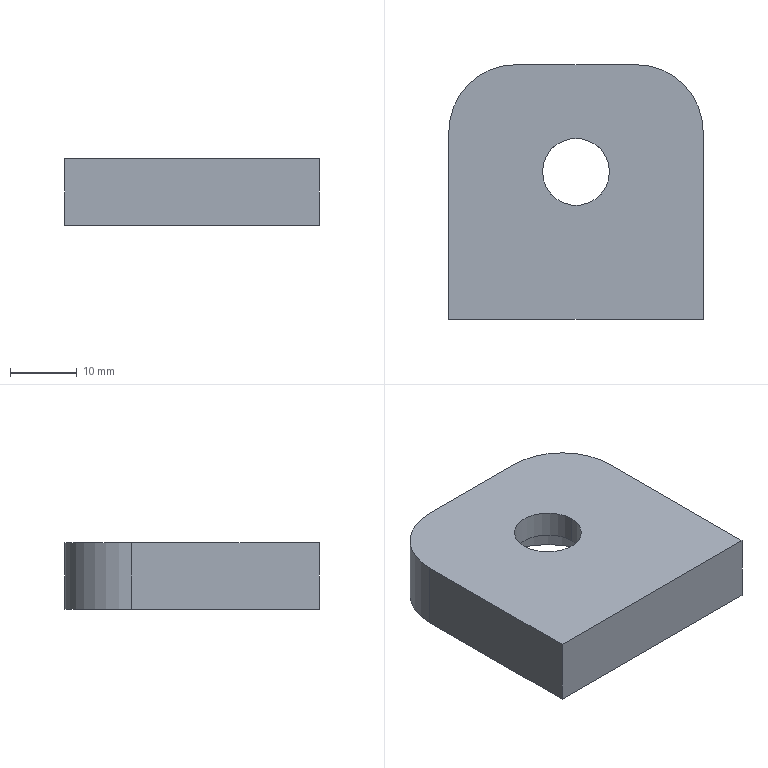Part | STEP file | Fixed block QY-1-06 | 1 solid | 13 faces | box 38 x 38 x 10 mm | volume 11416 mm3 | plane 7 | cylinder 6 | commonest cylinder face diameters 10 x2 20 x2 22 x2
STEP:
#1=CARTESIAN_POINT('',(0.,0.,0.));
#2=DIRECTION('',(0.,0.,1.));
#3=DIRECTION('',(1.,0.,0.));
#4=AXIS2_PLACEMENT_3D('',#1,#2,#3);
#5=CARTESIAN_POINT('',(-11.,3.,6.));
#6=VERTEX_POINT('',#5);
#7=CARTESIAN_POINT('',(-11.,3.,0.));
#8=VERTEX_POINT('',#7);
#9=CARTESIAN_POINT('',(-11.,3.,6.));
#10=DIRECTION('',(0.,0.,-1.));
#11=VECTOR('',#10,1.);
#12=LINE('',#9,#11);
#13=CARTESIAN_POINT('',(0.,3.,6.));
#14=DIRECTION('',(0.,0.,-1.));
#15=DIRECTION('',(-1.,0.,0.));
#16=AXIS2_PLACEMENT_3D('',#13,#14,#15);
#17=CYLINDRICAL_SURFACE('',#16,11.);
#18=CARTESIAN_POINT('',(6.283,0.));
#19=DIRECTION('',(0.,1.));
#20=VECTOR('',#19,1.);
#21=LINE('',#18,#20);
#22=(GEOMETRIC_REPRESENTATION_CONTEXT(2)PARAMETRIC_REPRESENTATION_CONTEXT()REPRESENTATION_CONTEXT('',''));
#23=DEFINITIONAL_REPRESENTATION('',(#21),#22);
#24=PCURVE('',#17,#23);
#25=CARTESIAN_POINT('',(0.,3.,6.));
#26=DIRECTION('',(0.,0.,-1.));
#27=DIRECTION('',(-1.,0.,0.));
#28=AXIS2_PLACEMENT_3D('',#25,#26,#27);
#29=CYLINDRICAL_SURFACE('',#28,11.);
#30=CARTESIAN_POINT('',(0.,0.));
#31=DIRECTION('',(0.,1.));
#32=VECTOR('',#31,1.);
#33=LINE('',#30,#32);
#34=(GEOMETRIC_REPRESENTATION_CONTEXT(2)PARAMETRIC_REPRESENTATION_CONTEXT()REPRESENTATION_CONTEXT('',''));
#35=DEFINITIONAL_REPRESENTATION('',(#33),#34);
#36=PCURVE('',#29,#35);
#37=SURFACE_CURVE('',#12,(#24,#36),.PCURVE_S1.);
#38=EDGE_CURVE('',#6,#8,#37,.T.);
#39=ORIENTED_EDGE('',*,*,#38,.T.);
#40=CARTESIAN_POINT('',(11.,3.,0.));
#41=VERTEX_POINT('',#40);
#42=CARTESIAN_POINT('',(0.,3.,0.));
#43=DIRECTION('',(0.,0.,-1.));
#44=DIRECTION('',(-1.,0.,0.));
#45=AXIS2_PLACEMENT_3D('',#42,#43,#44);
#46=CIRCLE('',#45,11.);
#47=CARTESIAN_POINT('',(0.,6.));
#48=DIRECTION('',(1.,0.));
#49=VECTOR('',#48,1.);
#50=LINE('',#47,#49);
#51=(GEOMETRIC_REPRESENTATION_CONTEXT(2)PARAMETRIC_REPRESENTATION_CONTEXT()REPRESENTATION_CONTEXT('',''));
#52=DEFINITIONAL_REPRESENTATION('',(#50),#51);
#53=PCURVE('',#17,#52);
#54=CARTESIAN_POINT('',(-9.,9.,0.));
#55=DIRECTION('',(0.,0.,1.));
#56=DIRECTION('',(1.,0.,0.));
#57=AXIS2_PLACEMENT_3D('',#54,#55,#56);
#58=PLANE('',#57);
#59=CARTESIAN_POINT('',(-2.,-6.));
#60=CARTESIAN_POINT('',(-2.,13.053));
#61=CARTESIAN_POINT('',(14.5,3.526));
#62=CARTESIAN_POINT('',(31.,-6.));
#63=CARTESIAN_POINT('',(14.5,-15.526));
#64=CARTESIAN_POINT('',(-2.,-25.053));
#65=CARTESIAN_POINT('',(-2.,-6.));
#66=(BOUNDED_CURVE()B_SPLINE_CURVE(2,(#59,#60,#61,#62,#63,#64,#65),.UNSPECIFIED.,.T.,.F.)B_SPLINE_CURVE_WITH_KNOTS((1,2,2,2,2,1),(-2.094,0.,2.094,4.189,6.283,8.378),.UNSPECIFIED.)CURVE()GEOMETRIC_REPRESENTATION_ITEM()RATIONAL_B_SPLINE_CURVE((1.,0.5,1.,0.5,1.,0.5,1.))REPRESENTATION_ITEM(''));
#67=(GEOMETRIC_REPRESENTATION_CONTEXT(2)PARAMETRIC_REPRESENTATION_CONTEXT()REPRESENTATION_CONTEXT('',''));
#68=DEFINITIONAL_REPRESENTATION('',(#66),#67);
#69=PCURVE('',#58,#68);
#70=SURFACE_CURVE('',#46,(#53,#69),.PCURVE_S1.);
#71=EDGE_CURVE('',#41,#8,#70,.T.);
#72=ORIENTED_EDGE('',*,*,#71,.F.);
#73=CARTESIAN_POINT('',(11.,3.,6.));
#74=VERTEX_POINT('',#73);
#75=CARTESIAN_POINT('',(11.,3.,6.));
#76=DIRECTION('',(0.,0.,-1.));
#77=VECTOR('',#76,1.);
#78=LINE('',#75,#77);
#79=CARTESIAN_POINT('',(3.142,0.));
#80=DIRECTION('',(0.,1.));
#81=VECTOR('',#80,1.);
#82=LINE('',#79,#81);
#83=(GEOMETRIC_REPRESENTATION_CONTEXT(2)PARAMETRIC_REPRESENTATION_CONTEXT()REPRESENTATION_CONTEXT('',''));
#84=DEFINITIONAL_REPRESENTATION('',(#82),#83);
#85=PCURVE('',#17,#84);
#86=CARTESIAN_POINT('',(3.142,0.));
#87=DIRECTION('',(0.,1.));
#88=VECTOR('',#87,1.);
#89=LINE('',#86,#88);
#90=(GEOMETRIC_REPRESENTATION_CONTEXT(2)PARAMETRIC_REPRESENTATION_CONTEXT()REPRESENTATION_CONTEXT('',''));
#91=DEFINITIONAL_REPRESENTATION('',(#89),#90);
#92=PCURVE('',#29,#91);
#93=SURFACE_CURVE('',#78,(#85,#92),.PCURVE_S1.);
#94=EDGE_CURVE('',#74,#41,#93,.T.);
#95=ORIENTED_EDGE('',*,*,#94,.F.);
#96=CARTESIAN_POINT('',(0.,3.,6.));
#97=DIRECTION('',(0.,0.,-1.));
#98=DIRECTION('',(-1.,0.,0.));
#99=AXIS2_PLACEMENT_3D('',#96,#97,#98);
#100=CIRCLE('',#99,11.);
#101=CARTESIAN_POINT('',(0.,0.));
#102=DIRECTION('',(1.,0.));
#103=VECTOR('',#102,1.);
#104=LINE('',#101,#103);
#105=(GEOMETRIC_REPRESENTATION_CONTEXT(2)PARAMETRIC_REPRESENTATION_CONTEXT()REPRESENTATION_CONTEXT('',''));
#106=DEFINITIONAL_REPRESENTATION('',(#104),#105);
#107=PCURVE('',#17,#106);
#108=CARTESIAN_POINT('',(0.,3.,6.));
#109=DIRECTION('',(0.,0.,-1.));
#110=DIRECTION('',(-1.,0.,0.));
#111=AXIS2_PLACEMENT_3D('',#108,#109,#110);
#112=PLANE('',#111);
#113=CARTESIAN_POINT('',(0.,0.));
#114=DIRECTION('',(1.,0.));
#115=AXIS2_PLACEMENT_2D('',#113,#114);
#116=CIRCLE('',#115,11.);
#117=(GEOMETRIC_REPRESENTATION_CONTEXT(2)PARAMETRIC_REPRESENTATION_CONTEXT()REPRESENTATION_CONTEXT('',''));
#118=DEFINITIONAL_REPRESENTATION('',(#116),#117);
#119=PCURVE('',#112,#118);
#120=SURFACE_CURVE('',#100,(#107,#119),.PCURVE_S1.);
#121=EDGE_CURVE('',#74,#6,#120,.T.);
#122=ORIENTED_EDGE('',*,*,#121,.T.);
#123=EDGE_LOOP('',(#39,#72,#95,#122));
#124=FACE_BOUND('',#123,.F.);
#125=ADVANCED_FACE('',(#124),#17,.F.);
#126=CARTESIAN_POINT('',(5.,3.,6.));
#127=VERTEX_POINT('',#126);
#128=CARTESIAN_POINT('',(5.,3.,10.));
#129=VERTEX_POINT('',#128);
#130=CARTESIAN_POINT('',(5.,3.,0.));
#131=DIRECTION('',(0.,0.,1.));
#132=VECTOR('',#131,1.);
#133=LINE('',#130,#132);
#134=CARTESIAN_POINT('',(0.,3.,0.));
#135=DIRECTION('',(0.,0.,1.));
#136=DIRECTION('',(1.,0.,0.));
#137=AXIS2_PLACEMENT_3D('',#134,#135,#136);
#138=CYLINDRICAL_SURFACE('',#137,5.);
#139=CARTESIAN_POINT('',(6.283,0.));
#140=DIRECTION('',(0.,1.));
#141=VECTOR('',#140,1.);
#142=LINE('',#139,#141);
#143=(GEOMETRIC_REPRESENTATION_CONTEXT(2)PARAMETRIC_REPRESENTATION_CONTEXT()REPRESENTATION_CONTEXT('',''));
#144=DEFINITIONAL_REPRESENTATION('',(#142),#143);
#145=PCURVE('',#138,#144);
#146=CARTESIAN_POINT('',(0.,3.,0.));
#147=DIRECTION('',(0.,0.,1.));
#148=DIRECTION('',(1.,0.,0.));
#149=AXIS2_PLACEMENT_3D('',#146,#147,#148);
#150=CYLINDRICAL_SURFACE('',#149,5.);
#151=CARTESIAN_POINT('',(0.,0.));
#152=DIRECTION('',(0.,1.));
#153=VECTOR('',#152,1.);
#154=LINE('',#151,#153);
#155=(GEOMETRIC_REPRESENTATION_CONTEXT(2)PARAMETRIC_REPRESENTATION_CONTEXT()REPRESENTATION_CONTEXT('',''));
#156=DEFINITIONAL_REPRESENTATION('',(#154),#155);
#157=PCURVE('',#150,#156);
#158=SURFACE_CURVE('',#133,(#145,#157),.PCURVE_S1.);
#159=EDGE_CURVE('',#127,#129,#158,.T.);
#160=ORIENTED_EDGE('',*,*,#159,.T.);
#161=CARTESIAN_POINT('',(-5.,3.,10.));
#162=VERTEX_POINT('',#161);
#163=CARTESIAN_POINT('',(0.,3.,10.));
#164=DIRECTION('',(0.,0.,1.));
#165=DIRECTION('',(1.,0.,0.));
#166=AXIS2_PLACEMENT_3D('',#163,#164,#165);
#167=CIRCLE('',#166,5.);
#168=CARTESIAN_POINT('',(0.,10.));
#169=DIRECTION('',(1.,0.));
#170=VECTOR('',#169,1.);
#171=LINE('',#168,#170);
#172=(GEOMETRIC_REPRESENTATION_CONTEXT(2)PARAMETRIC_REPRESENTATION_CONTEXT()REPRESENTATION_CONTEXT('',''));
#173=DEFINITIONAL_REPRESENTATION('',(#171),#172);
#174=PCURVE('',#138,#173);
#175=CARTESIAN_POINT('',(-9.,9.,10.));
#176=DIRECTION('',(0.,0.,1.));
#177=DIRECTION('',(1.,0.,0.));
#178=AXIS2_PLACEMENT_3D('',#175,#176,#177);
#179=PLANE('',#178);
#180=CARTESIAN_POINT('',(9.,-6.));
#181=DIRECTION('',(1.,0.));
#182=AXIS2_PLACEMENT_2D('',#180,#181);
#183=CIRCLE('',#182,5.);
#184=(GEOMETRIC_REPRESENTATION_CONTEXT(2)PARAMETRIC_REPRESENTATION_CONTEXT()REPRESENTATION_CONTEXT('',''));
#185=DEFINITIONAL_REPRESENTATION('',(#183),#184);
#186=PCURVE('',#179,#185);
#187=SURFACE_CURVE('',#167,(#174,#186),.PCURVE_S1.);
#188=EDGE_CURVE('',#162,#129,#187,.T.);
#189=ORIENTED_EDGE('',*,*,#188,.F.);
#190=CARTESIAN_POINT('',(-5.,3.,6.));
#191=VERTEX_POINT('',#190);
#192=CARTESIAN_POINT('',(-5.,3.,0.));
#193=DIRECTION('',(0.,0.,1.));
#194=VECTOR('',#193,1.);
#195=LINE('',#192,#194);
#196=CARTESIAN_POINT('',(3.142,0.));
#197=DIRECTION('',(0.,1.));
#198=VECTOR('',#197,1.);
#199=LINE('',#196,#198);
#200=(GEOMETRIC_REPRESENTATION_CONTEXT(2)PARAMETRIC_REPRESENTATION_CONTEXT()REPRESENTATION_CONTEXT('',''));
#201=DEFINITIONAL_REPRESENTATION('',(#199),#200);
#202=PCURVE('',#138,#201);
#203=CARTESIAN_POINT('',(3.142,0.));
#204=DIRECTION('',(0.,1.));
#205=VECTOR('',#204,1.);
#206=LINE('',#203,#205);
#207=(GEOMETRIC_REPRESENTATION_CONTEXT(2)PARAMETRIC_REPRESENTATION_CONTEXT()REPRESENTATION_CONTEXT('',''));
#208=DEFINITIONAL_REPRESENTATION('',(#206),#207);
#209=PCURVE('',#150,#208);
#210=SURFACE_CURVE('',#195,(#202,#209),.PCURVE_S1.);
#211=EDGE_CURVE('',#191,#162,#210,.T.);
#212=ORIENTED_EDGE('',*,*,#211,.F.);
#213=CARTESIAN_POINT('',(0.,3.,6.));
#214=DIRECTION('',(0.,0.,1.));
#215=DIRECTION('',(-1.,0.,0.));
#216=AXIS2_PLACEMENT_3D('',#213,#214,#215);
#217=CIRCLE('',#216,5.);
#218=CARTESIAN_POINT('',(3.142,6.));
#219=DIRECTION('',(1.,0.));
#220=VECTOR('',#219,1.);
#221=LINE('',#218,#220);
#222=(GEOMETRIC_REPRESENTATION_CONTEXT(2)PARAMETRIC_REPRESENTATION_CONTEXT()REPRESENTATION_CONTEXT('',''));
#223=DEFINITIONAL_REPRESENTATION('',(#221),#222);
#224=PCURVE('',#138,#223);
#225=CARTESIAN_POINT('',(5.,0.));
#226=CARTESIAN_POINT('',(5.,-8.66));
#227=CARTESIAN_POINT('',(-2.5,-4.33));
#228=CARTESIAN_POINT('',(-10.,0.));
#229=CARTESIAN_POINT('',(-2.5,4.33));
#230=CARTESIAN_POINT('',(5.,8.66));
#231=CARTESIAN_POINT('',(5.,0.));
#232=(BOUNDED_CURVE()B_SPLINE_CURVE(2,(#225,#226,#227,#228,#229,#230,#231),.UNSPECIFIED.,.T.,.F.)B_SPLINE_CURVE_WITH_KNOTS((1,2,2,2,2,1),(-2.094,0.,2.094,4.189,6.283,8.378),.UNSPECIFIED.)CURVE()GEOMETRIC_REPRESENTATION_ITEM()RATIONAL_B_SPLINE_CURVE((1.,0.5,1.,0.5,1.,0.5,1.))REPRESENTATION_ITEM(''));
#233=(GEOMETRIC_REPRESENTATION_CONTEXT(2)PARAMETRIC_REPRESENTATION_CONTEXT()REPRESENTATION_CONTEXT('',''));
#234=DEFINITIONAL_REPRESENTATION('',(#232),#233);
#235=PCURVE('',#112,#234);
#236=SURFACE_CURVE('',#217,(#224,#235),.PCURVE_S1.);
#237=EDGE_CURVE('',#191,#127,#236,.T.);
#238=ORIENTED_EDGE('',*,*,#237,.T.);
#239=EDGE_LOOP('',(#160,#189,#212,#238));
#240=FACE_BOUND('',#239,.F.);
#241=ADVANCED_FACE('',(#240),#138,.F.);
#242=CARTESIAN_POINT('',(0.,3.,10.));
#243=DIRECTION('',(0.,0.,1.));
#244=DIRECTION('',(1.,0.,0.));
#245=AXIS2_PLACEMENT_3D('',#242,#243,#244);
#246=CIRCLE('',#245,5.);
#247=CARTESIAN_POINT('',(0.,10.));
#248=DIRECTION('',(1.,0.));
#249=VECTOR('',#248,1.);
#250=LINE('',#247,#249);
#251=(GEOMETRIC_REPRESENTATION_CONTEXT(2)PARAMETRIC_REPRESENTATION_CONTEXT()REPRESENTATION_CONTEXT('',''));
#252=DEFINITIONAL_REPRESENTATION('',(#250),#251);
#253=PCURVE('',#150,#252);
#254=CARTESIAN_POINT('',(9.,-6.));
#255=DIRECTION('',(1.,0.));
#256=AXIS2_PLACEMENT_2D('',#254,#255);
#257=CIRCLE('',#256,5.);
#258=(GEOMETRIC_REPRESENTATION_CONTEXT(2)PARAMETRIC_REPRESENTATION_CONTEXT()REPRESENTATION_CONTEXT('',''));
#259=DEFINITIONAL_REPRESENTATION('',(#257),#258);
#260=PCURVE('',#179,#259);
#261=SURFACE_CURVE('',#246,(#253,#260),.PCURVE_S1.);
#262=EDGE_CURVE('',#129,#162,#261,.T.);
#263=ORIENTED_EDGE('',*,*,#262,.F.);
#264=ORIENTED_EDGE('',*,*,#159,.F.);
#265=CARTESIAN_POINT('',(0.,3.,6.));
#266=DIRECTION('',(0.,0.,1.));
#267=DIRECTION('',(-1.,0.,0.));
#268=AXIS2_PLACEMENT_3D('',#265,#266,#267);
#269=CIRCLE('',#268,5.);
#270=CARTESIAN_POINT('',(-3.142,6.));
#271=DIRECTION('',(1.,0.));
#272=VECTOR('',#271,1.);
#273=LINE('',#270,#272);
#274=(GEOMETRIC_REPRESENTATION_CONTEXT(2)PARAMETRIC_REPRESENTATION_CONTEXT()REPRESENTATION_CONTEXT('',''));
#275=DEFINITIONAL_REPRESENTATION('',(#273),#274);
#276=PCURVE('',#150,#275);
#277=CARTESIAN_POINT('',(5.,0.));
#278=CARTESIAN_POINT('',(5.,-8.66));
#279=CARTESIAN_POINT('',(-2.5,-4.33));
#280=CARTESIAN_POINT('',(-10.,0.));
#281=CARTESIAN_POINT('',(-2.5,4.33));
#282=CARTESIAN_POINT('',(5.,8.66));
#283=CARTESIAN_POINT('',(5.,0.));
#284=(BOUNDED_CURVE()B_SPLINE_CURVE(2,(#277,#278,#279,#280,#281,#282,#283),.UNSPECIFIED.,.T.,.F.)B_SPLINE_CURVE_WITH_KNOTS((1,2,2,2,2,1),(-2.094,0.,2.094,4.189,6.283,8.378),.UNSPECIFIED.)CURVE()GEOMETRIC_REPRESENTATION_ITEM()RATIONAL_B_SPLINE_CURVE((1.,0.5,1.,0.5,1.,0.5,1.))REPRESENTATION_ITEM(''));
#285=(GEOMETRIC_REPRESENTATION_CONTEXT(2)PARAMETRIC_REPRESENTATION_CONTEXT()REPRESENTATION_CONTEXT('',''));
#286=DEFINITIONAL_REPRESENTATION('',(#284),#285);
#287=PCURVE('',#112,#286);
#288=SURFACE_CURVE('',#269,(#276,#287),.PCURVE_S1.);
#289=EDGE_CURVE('',#127,#191,#288,.T.);
#290=ORIENTED_EDGE('',*,*,#289,.T.);
#291=ORIENTED_EDGE('',*,*,#211,.T.);
#292=EDGE_LOOP('',(#263,#264,#290,#291));
#293=FACE_BOUND('',#292,.F.);
#294=ADVANCED_FACE('',(#293),#150,.F.);
#295=CARTESIAN_POINT('',(19.,-19.,0.));
#296=VERTEX_POINT('',#295);
#297=CARTESIAN_POINT('',(19.,9.,0.));
#298=VERTEX_POINT('',#297);
#299=CARTESIAN_POINT('',(19.,9.,0.));
#300=DIRECTION('',(0.,1.,0.));
#301=VECTOR('',#300,1.);
#302=LINE('',#299,#301);
#303=CARTESIAN_POINT('',(19.,9.,10.));
#304=DIRECTION('',(-1.,0.,0.));
#305=DIRECTION('',(0.,-1.,0.));
#306=AXIS2_PLACEMENT_3D('',#303,#304,#305);
#307=PLANE('',#306);
#308=CARTESIAN_POINT('',(0.,-10.));
#309=DIRECTION('',(-1.,0.));
#310=VECTOR('',#309,1.);
#311=LINE('',#308,#310);
#312=(GEOMETRIC_REPRESENTATION_CONTEXT(2)PARAMETRIC_REPRESENTATION_CONTEXT()REPRESENTATION_CONTEXT('',''));
#313=DEFINITIONAL_REPRESENTATION('',(#311),#312);
#314=PCURVE('',#307,#313);
#315=CARTESIAN_POINT('',(28.,0.));
#316=DIRECTION('',(0.,1.));
#317=VECTOR('',#316,1.);
#318=LINE('',#315,#317);
#319=(GEOMETRIC_REPRESENTATION_CONTEXT(2)PARAMETRIC_REPRESENTATION_CONTEXT()REPRESENTATION_CONTEXT('',''));
#320=DEFINITIONAL_REPRESENTATION('',(#318),#319);
#321=PCURVE('',#58,#320);
#322=SURFACE_CURVE('',#302,(#314,#321),.PCURVE_S1.);
#323=EDGE_CURVE('',#296,#298,#322,.T.);
#324=ORIENTED_EDGE('',*,*,#323,.T.);
#325=CARTESIAN_POINT('',(19.,9.,10.));
#326=VERTEX_POINT('',#325);
#327=CARTESIAN_POINT('',(19.,9.,10.));
#328=DIRECTION('',(0.,0.,-1.));
#329=VECTOR('',#328,1.);
#330=LINE('',#327,#329);
#331=CARTESIAN_POINT('',(0.,0.));
#332=DIRECTION('',(0.,-1.));
#333=VECTOR('',#332,1.);
#334=LINE('',#331,#333);
#335=(GEOMETRIC_REPRESENTATION_CONTEXT(2)PARAMETRIC_REPRESENTATION_CONTEXT()REPRESENTATION_CONTEXT('',''));
#336=DEFINITIONAL_REPRESENTATION('',(#334),#335);
#337=PCURVE('',#307,#336);
#338=CARTESIAN_POINT('',(9.,9.,10.));
#339=DIRECTION('',(0.,0.,-1.));
#340=DIRECTION('',(-1.,0.,0.));
#341=AXIS2_PLACEMENT_3D('',#338,#339,#340);
#342=CYLINDRICAL_SURFACE('',#341,10.);
#343=CARTESIAN_POINT('',(3.142,0.));
#344=DIRECTION('',(0.,1.));
#345=VECTOR('',#344,1.);
#346=LINE('',#343,#345);
#347=(GEOMETRIC_REPRESENTATION_CONTEXT(2)PARAMETRIC_REPRESENTATION_CONTEXT()REPRESENTATION_CONTEXT('',''));
#348=DEFINITIONAL_REPRESENTATION('',(#346),#347);
#349=PCURVE('',#342,#348);
#350=SURFACE_CURVE('',#330,(#337,#349),.PCURVE_S1.);
#351=EDGE_CURVE('',#326,#298,#350,.T.);
#352=ORIENTED_EDGE('',*,*,#351,.F.);
#353=CARTESIAN_POINT('',(19.,-19.,10.));
#354=VERTEX_POINT('',#353);
#355=CARTESIAN_POINT('',(19.,9.,10.));
#356=DIRECTION('',(0.,1.,0.));
#357=VECTOR('',#356,1.);
#358=LINE('',#355,#357);
#359=CARTESIAN_POINT('',(0.,0.));
#360=DIRECTION('',(-1.,0.));
#361=VECTOR('',#360,1.);
#362=LINE('',#359,#361);
#363=(GEOMETRIC_REPRESENTATION_CONTEXT(2)PARAMETRIC_REPRESENTATION_CONTEXT()REPRESENTATION_CONTEXT('',''));
#364=DEFINITIONAL_REPRESENTATION('',(#362),#363);
#365=PCURVE('',#307,#364);
#366=CARTESIAN_POINT('',(28.,0.));
#367=DIRECTION('',(0.,1.));
#368=VECTOR('',#367,1.);
#369=LINE('',#366,#368);
#370=(GEOMETRIC_REPRESENTATION_CONTEXT(2)PARAMETRIC_REPRESENTATION_CONTEXT()REPRESENTATION_CONTEXT('',''));
#371=DEFINITIONAL_REPRESENTATION('',(#369),#370);
#372=PCURVE('',#179,#371);
#373=SURFACE_CURVE('',#358,(#365,#372),.PCURVE_S1.);
#374=EDGE_CURVE('',#354,#326,#373,.T.);
#375=ORIENTED_EDGE('',*,*,#374,.F.);
#376=CARTESIAN_POINT('',(19.,-19.,10.));
#377=DIRECTION('',(0.,0.,-1.));
#378=VECTOR('',#377,1.);
#379=LINE('',#376,#378);
#380=CARTESIAN_POINT('',(28.,0.));
#381=DIRECTION('',(0.,-1.));
#382=VECTOR('',#381,1.);
#383=LINE('',#380,#382);
#384=(GEOMETRIC_REPRESENTATION_CONTEXT(2)PARAMETRIC_REPRESENTATION_CONTEXT()REPRESENTATION_CONTEXT('',''));
#385=DEFINITIONAL_REPRESENTATION('',(#383),#384);
#386=PCURVE('',#307,#385);
#387=CARTESIAN_POINT('',(-19.,-19.,10.));
#388=DIRECTION('',(0.,1.,0.));
#389=DIRECTION('',(0.,0.,1.));
#390=AXIS2_PLACEMENT_3D('',#387,#388,#389);
#391=PLANE('',#390);
#392=CARTESIAN_POINT('',(0.,38.));
#393=DIRECTION('',(-1.,0.));
#394=VECTOR('',#393,1.);
#395=LINE('',#392,#394);
#396=(GEOMETRIC_REPRESENTATION_CONTEXT(2)PARAMETRIC_REPRESENTATION_CONTEXT()REPRESENTATION_CONTEXT('',''));
#397=DEFINITIONAL_REPRESENTATION('',(#395),#396);
#398=PCURVE('',#391,#397);
#399=SURFACE_CURVE('',#379,(#386,#398),.PCURVE_S1.);
#400=EDGE_CURVE('',#354,#296,#399,.T.);
#401=ORIENTED_EDGE('',*,*,#400,.T.);
#402=EDGE_LOOP('',(#324,#352,#375,#401));
#403=FACE_BOUND('',#402,.T.);
#404=ADVANCED_FACE('',(#403),#307,.F.);
#405=CARTESIAN_POINT('',(9.,19.,0.));
#406=VERTEX_POINT('',#405);
#407=CARTESIAN_POINT('',(9.,9.,0.));
#408=DIRECTION('',(0.,0.,1.));
#409=DIRECTION('',(-1.,0.,0.));
#410=AXIS2_PLACEMENT_3D('',#407,#408,#409);
#411=CIRCLE('',#410,10.);
#412=CARTESIAN_POINT('',(6.283,10.));
#413=DIRECTION('',(-1.,0.));
#414=VECTOR('',#413,1.);
#415=LINE('',#412,#414);
#416=(GEOMETRIC_REPRESENTATION_CONTEXT(2)PARAMETRIC_REPRESENTATION_CONTEXT()REPRESENTATION_CONTEXT('',''));
#417=DEFINITIONAL_REPRESENTATION('',(#415),#416);
#418=PCURVE('',#342,#417);
#419=CARTESIAN_POINT('',(18.,0.));
#420=DIRECTION('',(-1.,0.));
#421=AXIS2_PLACEMENT_2D('',#419,#420);
#422=CIRCLE('',#421,10.);
#423=(GEOMETRIC_REPRESENTATION_CONTEXT(2)PARAMETRIC_REPRESENTATION_CONTEXT()REPRESENTATION_CONTEXT('',''));
#424=DEFINITIONAL_REPRESENTATION('',(#422),#423);
#425=PCURVE('',#58,#424);
#426=SURFACE_CURVE('',#411,(#418,#425),.PCURVE_S1.);
#427=EDGE_CURVE('',#298,#406,#426,.T.);
#428=ORIENTED_EDGE('',*,*,#427,.T.);
#429=CARTESIAN_POINT('',(9.,19.,10.));
#430=VERTEX_POINT('',#429);
#431=CARTESIAN_POINT('',(9.,19.,10.));
#432=DIRECTION('',(0.,0.,-1.));
#433=VECTOR('',#432,1.);
#434=LINE('',#431,#433);
#435=CARTESIAN_POINT('',(1.571,0.));
#436=DIRECTION('',(0.,1.));
#437=VECTOR('',#436,1.);
#438=LINE('',#435,#437);
#439=(GEOMETRIC_REPRESENTATION_CONTEXT(2)PARAMETRIC_REPRESENTATION_CONTEXT()REPRESENTATION_CONTEXT('',''));
#440=DEFINITIONAL_REPRESENTATION('',(#438),#439);
#441=PCURVE('',#342,#440);
#442=CARTESIAN_POINT('',(-9.,19.,10.));
#443=DIRECTION('',(0.,-1.,0.));
#444=DIRECTION('',(1.,0.,0.));
#445=AXIS2_PLACEMENT_3D('',#442,#443,#444);
#446=PLANE('',#445);
#447=CARTESIAN_POINT('',(18.,0.));
#448=DIRECTION('',(0.,-1.));
#449=VECTOR('',#448,1.);
#450=LINE('',#447,#449);
#451=(GEOMETRIC_REPRESENTATION_CONTEXT(2)PARAMETRIC_REPRESENTATION_CONTEXT()REPRESENTATION_CONTEXT('',''));
#452=DEFINITIONAL_REPRESENTATION('',(#450),#451);
#453=PCURVE('',#446,#452);
#454=SURFACE_CURVE('',#434,(#441,#453),.PCURVE_S1.);
#455=EDGE_CURVE('',#430,#406,#454,.T.);
#456=ORIENTED_EDGE('',*,*,#455,.F.);
#457=CARTESIAN_POINT('',(9.,9.,10.));
#458=DIRECTION('',(0.,0.,1.));
#459=DIRECTION('',(-1.,0.,0.));
#460=AXIS2_PLACEMENT_3D('',#457,#458,#459);
#461=CIRCLE('',#460,10.);
#462=CARTESIAN_POINT('',(6.283,0.));
#463=DIRECTION('',(-1.,0.));
#464=VECTOR('',#463,1.);
#465=LINE('',#462,#464);
#466=(GEOMETRIC_REPRESENTATION_CONTEXT(2)PARAMETRIC_REPRESENTATION_CONTEXT()REPRESENTATION_CONTEXT('',''));
#467=DEFINITIONAL_REPRESENTATION('',(#465),#466);
#468=PCURVE('',#342,#467);
#469=CARTESIAN_POINT('',(18.,0.));
#470=DIRECTION('',(-1.,0.));
#471=AXIS2_PLACEMENT_2D('',#469,#470);
#472=CIRCLE('',#471,10.);
#473=(GEOMETRIC_REPRESENTATION_CONTEXT(2)PARAMETRIC_REPRESENTATION_CONTEXT()REPRESENTATION_CONTEXT('',''));
#474=DEFINITIONAL_REPRESENTATION('',(#472),#473);
#475=PCURVE('',#179,#474);
#476=SURFACE_CURVE('',#461,(#468,#475),.PCURVE_S1.);
#477=EDGE_CURVE('',#326,#430,#476,.T.);
#478=ORIENTED_EDGE('',*,*,#477,.F.);
#479=ORIENTED_EDGE('',*,*,#351,.T.);
#480=EDGE_LOOP('',(#428,#456,#478,#479));
#481=FACE_BOUND('',#480,.T.);
#482=ADVANCED_FACE('',(#481),#342,.T.);
#483=CARTESIAN_POINT('',(-9.,19.,0.));
#484=VERTEX_POINT('',#483);
#485=CARTESIAN_POINT('',(-9.,19.,0.));
#486=DIRECTION('',(-1.,0.,0.));
#487=VECTOR('',#486,1.);
#488=LINE('',#485,#487);
#489=CARTESIAN_POINT('',(0.,-10.));
#490=DIRECTION('',(-1.,0.));
#491=VECTOR('',#490,1.);
#492=LINE('',#489,#491);
#493=(GEOMETRIC_REPRESENTATION_CONTEXT(2)PARAMETRIC_REPRESENTATION_CONTEXT()REPRESENTATION_CONTEXT('',''));
#494=DEFINITIONAL_REPRESENTATION('',(#492),#493);
#495=PCURVE('',#446,#494);
#496=CARTESIAN_POINT('',(0.,10.));
#497=DIRECTION('',(-1.,0.));
#498=VECTOR('',#497,1.);
#499=LINE('',#496,#498);
#500=(GEOMETRIC_REPRESENTATION_CONTEXT(2)PARAMETRIC_REPRESENTATION_CONTEXT()REPRESENTATION_CONTEXT('',''));
#501=DEFINITIONAL_REPRESENTATION('',(#499),#500);
#502=PCURVE('',#58,#501);
#503=SURFACE_CURVE('',#488,(#495,#502),.PCURVE_S1.);
#504=EDGE_CURVE('',#406,#484,#503,.T.);
#505=ORIENTED_EDGE('',*,*,#504,.T.);
#506=CARTESIAN_POINT('',(-9.,19.,10.));
#507=VERTEX_POINT('',#506);
#508=CARTESIAN_POINT('',(-9.,19.,10.));
#509=DIRECTION('',(0.,0.,-1.));
#510=VECTOR('',#509,1.);
#511=LINE('',#508,#510);
#512=CARTESIAN_POINT('',(0.,0.));
#513=DIRECTION('',(0.,-1.));
#514=VECTOR('',#513,1.);
#515=LINE('',#512,#514);
#516=(GEOMETRIC_REPRESENTATION_CONTEXT(2)PARAMETRIC_REPRESENTATION_CONTEXT()REPRESENTATION_CONTEXT('',''));
#517=DEFINITIONAL_REPRESENTATION('',(#515),#516);
#518=PCURVE('',#446,#517);
#519=CARTESIAN_POINT('',(-9.,9.,10.));
#520=DIRECTION('',(0.,0.,-1.));
#521=DIRECTION('',(-1.,0.,0.));
#522=AXIS2_PLACEMENT_3D('',#519,#520,#521);
#523=CYLINDRICAL_SURFACE('',#522,10.);
#524=CARTESIAN_POINT('',(1.571,0.));
#525=DIRECTION('',(0.,1.));
#526=VECTOR('',#525,1.);
#527=LINE('',#524,#526);
#528=(GEOMETRIC_REPRESENTATION_CONTEXT(2)PARAMETRIC_REPRESENTATION_CONTEXT()REPRESENTATION_CONTEXT('',''));
#529=DEFINITIONAL_REPRESENTATION('',(#527),#528);
#530=PCURVE('',#523,#529);
#531=SURFACE_CURVE('',#511,(#518,#530),.PCURVE_S1.);
#532=EDGE_CURVE('',#507,#484,#531,.T.);
#533=ORIENTED_EDGE('',*,*,#532,.F.);
#534=CARTESIAN_POINT('',(-9.,19.,10.));
#535=DIRECTION('',(-1.,0.,0.));
#536=VECTOR('',#535,1.);
#537=LINE('',#534,#536);
#538=CARTESIAN_POINT('',(0.,0.));
#539=DIRECTION('',(-1.,0.));
#540=VECTOR('',#539,1.);
#541=LINE('',#538,#540);
#542=(GEOMETRIC_REPRESENTATION_CONTEXT(2)PARAMETRIC_REPRESENTATION_CONTEXT()REPRESENTATION_CONTEXT('',''));
#543=DEFINITIONAL_REPRESENTATION('',(#541),#542);
#544=PCURVE('',#446,#543);
#545=CARTESIAN_POINT('',(0.,10.));
#546=DIRECTION('',(-1.,0.));
#547=VECTOR('',#546,1.);
#548=LINE('',#545,#547);
#549=(GEOMETRIC_REPRESENTATION_CONTEXT(2)PARAMETRIC_REPRESENTATION_CONTEXT()REPRESENTATION_CONTEXT('',''));
#550=DEFINITIONAL_REPRESENTATION('',(#548),#549);
#551=PCURVE('',#179,#550);
#552=SURFACE_CURVE('',#537,(#544,#551),.PCURVE_S1.);
#553=EDGE_CURVE('',#430,#507,#552,.T.);
#554=ORIENTED_EDGE('',*,*,#553,.F.);
#555=ORIENTED_EDGE('',*,*,#455,.T.);
#556=EDGE_LOOP('',(#505,#533,#554,#555));
#557=FACE_BOUND('',#556,.T.);
#558=ADVANCED_FACE('',(#557),#446,.F.);
#559=CARTESIAN_POINT('',(-19.,9.,0.));
#560=VERTEX_POINT('',#559);
#561=CARTESIAN_POINT('',(-9.,9.,0.));
#562=DIRECTION('',(0.,0.,1.));
#563=DIRECTION('',(1.,0.,0.));
#564=AXIS2_PLACEMENT_3D('',#561,#562,#563);
#565=CIRCLE('',#564,10.);
#566=CARTESIAN_POINT('',(3.142,10.));
#567=DIRECTION('',(-1.,0.));
#568=VECTOR('',#567,1.);
#569=LINE('',#566,#568);
#570=(GEOMETRIC_REPRESENTATION_CONTEXT(2)PARAMETRIC_REPRESENTATION_CONTEXT()REPRESENTATION_CONTEXT('',''));
#571=DEFINITIONAL_REPRESENTATION('',(#569),#570);
#572=PCURVE('',#523,#571);
#573=CARTESIAN_POINT('',(0.,0.));
#574=DIRECTION('',(1.,0.));
#575=AXIS2_PLACEMENT_2D('',#573,#574);
#576=CIRCLE('',#575,10.);
#577=(GEOMETRIC_REPRESENTATION_CONTEXT(2)PARAMETRIC_REPRESENTATION_CONTEXT()REPRESENTATION_CONTEXT('',''));
#578=DEFINITIONAL_REPRESENTATION('',(#576),#577);
#579=PCURVE('',#58,#578);
#580=SURFACE_CURVE('',#565,(#572,#579),.PCURVE_S1.);
#581=EDGE_CURVE('',#484,#560,#580,.T.);
#582=ORIENTED_EDGE('',*,*,#581,.T.);
#583=CARTESIAN_POINT('',(-19.,9.,10.));
#584=VERTEX_POINT('',#583);
#585=CARTESIAN_POINT('',(-19.,9.,10.));
#586=DIRECTION('',(0.,0.,-1.));
#587=VECTOR('',#586,1.);
#588=LINE('',#585,#587);
#589=CARTESIAN_POINT('',(0.,0.));
#590=DIRECTION('',(0.,1.));
#591=VECTOR('',#590,1.);
#592=LINE('',#589,#591);
#593=(GEOMETRIC_REPRESENTATION_CONTEXT(2)PARAMETRIC_REPRESENTATION_CONTEXT()REPRESENTATION_CONTEXT('',''));
#594=DEFINITIONAL_REPRESENTATION('',(#592),#593);
#595=PCURVE('',#523,#594);
#596=CARTESIAN_POINT('',(-19.,9.,10.));
#597=DIRECTION('',(1.,0.,0.));
#598=DIRECTION('',(0.,1.,0.));
#599=AXIS2_PLACEMENT_3D('',#596,#597,#598);
#600=PLANE('',#599);
#601=CARTESIAN_POINT('',(0.,0.));
#602=DIRECTION('',(0.,-1.));
#603=VECTOR('',#602,1.);
#604=LINE('',#601,#603);
#605=(GEOMETRIC_REPRESENTATION_CONTEXT(2)PARAMETRIC_REPRESENTATION_CONTEXT()REPRESENTATION_CONTEXT('',''));
#606=DEFINITIONAL_REPRESENTATION('',(#604),#605);
#607=PCURVE('',#600,#606);
#608=SURFACE_CURVE('',#588,(#595,#607),.PCURVE_S1.);
#609=EDGE_CURVE('',#584,#560,#608,.T.);
#610=ORIENTED_EDGE('',*,*,#609,.F.);
#611=CARTESIAN_POINT('',(-9.,9.,10.));
#612=DIRECTION('',(0.,0.,1.));
#613=DIRECTION('',(1.,0.,0.));
#614=AXIS2_PLACEMENT_3D('',#611,#612,#613);
#615=CIRCLE('',#614,10.);
#616=CARTESIAN_POINT('',(3.142,0.));
#617=DIRECTION('',(-1.,0.));
#618=VECTOR('',#617,1.);
#619=LINE('',#616,#618);
#620=(GEOMETRIC_REPRESENTATION_CONTEXT(2)PARAMETRIC_REPRESENTATION_CONTEXT()REPRESENTATION_CONTEXT('',''));
#621=DEFINITIONAL_REPRESENTATION('',(#619),#620);
#622=PCURVE('',#523,#621);
#623=CARTESIAN_POINT('',(0.,0.));
#624=DIRECTION('',(1.,0.));
#625=AXIS2_PLACEMENT_2D('',#623,#624);
#626=CIRCLE('',#625,10.);
#627=(GEOMETRIC_REPRESENTATION_CONTEXT(2)PARAMETRIC_REPRESENTATION_CONTEXT()REPRESENTATION_CONTEXT('',''));
#628=DEFINITIONAL_REPRESENTATION('',(#626),#627);
#629=PCURVE('',#179,#628);
#630=SURFACE_CURVE('',#615,(#622,#629),.PCURVE_S1.);
#631=EDGE_CURVE('',#507,#584,#630,.T.);
#632=ORIENTED_EDGE('',*,*,#631,.F.);
#633=ORIENTED_EDGE('',*,*,#532,.T.);
#634=EDGE_LOOP('',(#582,#610,#632,#633));
#635=FACE_BOUND('',#634,.T.);
#636=ADVANCED_FACE('',(#635),#523,.T.);
#637=CARTESIAN_POINT('',(-19.,-19.,0.));
#638=VERTEX_POINT('',#637);
#639=CARTESIAN_POINT('',(-19.,9.,0.));
#640=DIRECTION('',(0.,-1.,0.));
#641=VECTOR('',#640,1.);
#642=LINE('',#639,#641);
#643=CARTESIAN_POINT('',(0.,-10.));
#644=DIRECTION('',(-1.,0.));
#645=VECTOR('',#644,1.);
#646=LINE('',#643,#645);
#647=(GEOMETRIC_REPRESENTATION_CONTEXT(2)PARAMETRIC_REPRESENTATION_CONTEXT()REPRESENTATION_CONTEXT('',''));
#648=DEFINITIONAL_REPRESENTATION('',(#646),#647);
#649=PCURVE('',#600,#648);
#650=CARTESIAN_POINT('',(-10.,0.));
#651=DIRECTION('',(0.,-1.));
#652=VECTOR('',#651,1.);
#653=LINE('',#650,#652);
#654=(GEOMETRIC_REPRESENTATION_CONTEXT(2)PARAMETRIC_REPRESENTATION_CONTEXT()REPRESENTATION_CONTEXT('',''));
#655=DEFINITIONAL_REPRESENTATION('',(#653),#654);
#656=PCURVE('',#58,#655);
#657=SURFACE_CURVE('',#642,(#649,#656),.PCURVE_S1.);
#658=EDGE_CURVE('',#560,#638,#657,.T.);
#659=ORIENTED_EDGE('',*,*,#658,.T.);
#660=CARTESIAN_POINT('',(-19.,-19.,10.));
#661=VERTEX_POINT('',#660);
#662=CARTESIAN_POINT('',(-19.,-19.,10.));
#663=DIRECTION('',(0.,0.,-1.));
#664=VECTOR('',#663,1.);
#665=LINE('',#662,#664);
#666=CARTESIAN_POINT('',(-28.,0.));
#667=DIRECTION('',(0.,-1.));
#668=VECTOR('',#667,1.);
#669=LINE('',#666,#668);
#670=(GEOMETRIC_REPRESENTATION_CONTEXT(2)PARAMETRIC_REPRESENTATION_CONTEXT()REPRESENTATION_CONTEXT('',''));
#671=DEFINITIONAL_REPRESENTATION('',(#669),#670);
#672=PCURVE('',#600,#671);
#673=CARTESIAN_POINT('',(0.,0.));
#674=DIRECTION('',(-1.,0.));
#675=VECTOR('',#674,1.);
#676=LINE('',#673,#675);
#677=(GEOMETRIC_REPRESENTATION_CONTEXT(2)PARAMETRIC_REPRESENTATION_CONTEXT()REPRESENTATION_CONTEXT('',''));
#678=DEFINITIONAL_REPRESENTATION('',(#676),#677);
#679=PCURVE('',#391,#678);
#680=SURFACE_CURVE('',#665,(#672,#679),.PCURVE_S1.);
#681=EDGE_CURVE('',#661,#638,#680,.T.);
#682=ORIENTED_EDGE('',*,*,#681,.F.);
#683=CARTESIAN_POINT('',(-19.,9.,10.));
#684=DIRECTION('',(0.,-1.,0.));
#685=VECTOR('',#684,1.);
#686=LINE('',#683,#685);
#687=CARTESIAN_POINT('',(0.,0.));
#688=DIRECTION('',(-1.,0.));
#689=VECTOR('',#688,1.);
#690=LINE('',#687,#689);
#691=(GEOMETRIC_REPRESENTATION_CONTEXT(2)PARAMETRIC_REPRESENTATION_CONTEXT()REPRESENTATION_CONTEXT('',''));
#692=DEFINITIONAL_REPRESENTATION('',(#690),#691);
#693=PCURVE('',#600,#692);
#694=CARTESIAN_POINT('',(-10.,0.));
#695=DIRECTION('',(0.,-1.));
#696=VECTOR('',#695,1.);
#697=LINE('',#694,#696);
#698=(GEOMETRIC_REPRESENTATION_CONTEXT(2)PARAMETRIC_REPRESENTATION_CONTEXT()REPRESENTATION_CONTEXT('',''));
#699=DEFINITIONAL_REPRESENTATION('',(#697),#698);
#700=PCURVE('',#179,#699);
#701=SURFACE_CURVE('',#686,(#693,#700),.PCURVE_S1.);
#702=EDGE_CURVE('',#584,#661,#701,.T.);
#703=ORIENTED_EDGE('',*,*,#702,.F.);
#704=ORIENTED_EDGE('',*,*,#609,.T.);
#705=EDGE_LOOP('',(#659,#682,#703,#704));
#706=FACE_BOUND('',#705,.T.);
#707=ADVANCED_FACE('',(#706),#600,.F.);
#708=CARTESIAN_POINT('',(-19.,-19.,0.));
#709=DIRECTION('',(1.,0.,0.));
#710=VECTOR('',#709,1.);
#711=LINE('',#708,#710);
#712=CARTESIAN_POINT('',(-10.,0.));
#713=DIRECTION('',(0.,1.));
#714=VECTOR('',#713,1.);
#715=LINE('',#712,#714);
#716=(GEOMETRIC_REPRESENTATION_CONTEXT(2)PARAMETRIC_REPRESENTATION_CONTEXT()REPRESENTATION_CONTEXT('',''));
#717=DEFINITIONAL_REPRESENTATION('',(#715),#716);
#718=PCURVE('',#391,#717);
#719=CARTESIAN_POINT('',(-10.,-28.));
#720=DIRECTION('',(1.,0.));
#721=VECTOR('',#720,1.);
#722=LINE('',#719,#721);
#723=(GEOMETRIC_REPRESENTATION_CONTEXT(2)PARAMETRIC_REPRESENTATION_CONTEXT()REPRESENTATION_CONTEXT('',''));
#724=DEFINITIONAL_REPRESENTATION('',(#722),#723);
#725=PCURVE('',#58,#724);
#726=SURFACE_CURVE('',#711,(#718,#725),.PCURVE_S1.);
#727=EDGE_CURVE('',#638,#296,#726,.T.);
#728=ORIENTED_EDGE('',*,*,#727,.T.);
#729=ORIENTED_EDGE('',*,*,#400,.F.);
#730=CARTESIAN_POINT('',(-19.,-19.,10.));
#731=DIRECTION('',(1.,0.,0.));
#732=VECTOR('',#731,1.);
#733=LINE('',#730,#732);
#734=CARTESIAN_POINT('',(0.,0.));
#735=DIRECTION('',(0.,1.));
#736=VECTOR('',#735,1.);
#737=LINE('',#734,#736);
#738=(GEOMETRIC_REPRESENTATION_CONTEXT(2)PARAMETRIC_REPRESENTATION_CONTEXT()REPRESENTATION_CONTEXT('',''));
#739=DEFINITIONAL_REPRESENTATION('',(#737),#738);
#740=PCURVE('',#391,#739);
#741=CARTESIAN_POINT('',(-10.,-28.));
#742=DIRECTION('',(1.,0.));
#743=VECTOR('',#742,1.);
#744=LINE('',#741,#743);
#745=(GEOMETRIC_REPRESENTATION_CONTEXT(2)PARAMETRIC_REPRESENTATION_CONTEXT()REPRESENTATION_CONTEXT('',''));
#746=DEFINITIONAL_REPRESENTATION('',(#744),#745);
#747=PCURVE('',#179,#746);
#748=SURFACE_CURVE('',#733,(#740,#747),.PCURVE_S1.);
#749=EDGE_CURVE('',#661,#354,#748,.T.);
#750=ORIENTED_EDGE('',*,*,#749,.F.);
#751=ORIENTED_EDGE('',*,*,#681,.T.);
#752=EDGE_LOOP('',(#728,#729,#750,#751));
#753=FACE_BOUND('',#752,.T.);
#754=ADVANCED_FACE('',(#753),#391,.F.);
#755=ORIENTED_EDGE('',*,*,#262,.F.);
#756=ORIENTED_EDGE('',*,*,#188,.F.);
#757=EDGE_LOOP('',(#755,#756));
#758=FACE_BOUND('',#757,.T.);
#759=ORIENTED_EDGE('',*,*,#374,.T.);
#760=ORIENTED_EDGE('',*,*,#477,.T.);
#761=ORIENTED_EDGE('',*,*,#553,.T.);
#762=ORIENTED_EDGE('',*,*,#631,.T.);
#763=ORIENTED_EDGE('',*,*,#702,.T.);
#764=ORIENTED_EDGE('',*,*,#749,.T.);
#765=EDGE_LOOP('',(#759,#760,#761,#762,#763,#764));
#766=FACE_BOUND('',#765,.T.);
#767=ADVANCED_FACE('',(#758,#766),#179,.T.);
#768=CARTESIAN_POINT('',(0.,3.,0.));
#769=DIRECTION('',(0.,0.,-1.));
#770=DIRECTION('',(-1.,0.,0.));
#771=AXIS2_PLACEMENT_3D('',#768,#769,#770);
#772=CIRCLE('',#771,11.);
#773=CARTESIAN_POINT('',(-2.,-6.));
#774=CARTESIAN_POINT('',(-2.,13.053));
#775=CARTESIAN_POINT('',(14.5,3.526));
#776=CARTESIAN_POINT('',(31.,-6.));
#777=CARTESIAN_POINT('',(14.5,-15.526));
#778=CARTESIAN_POINT('',(-2.,-25.053));
#779=CARTESIAN_POINT('',(-2.,-6.));
#780=(BOUNDED_CURVE()B_SPLINE_CURVE(2,(#773,#774,#775,#776,#777,#778,#779),.UNSPECIFIED.,.T.,.F.)B_SPLINE_CURVE_WITH_KNOTS((1,2,2,2,2,1),(-2.094,0.,2.094,4.189,6.283,8.378),.UNSPECIFIED.)CURVE()GEOMETRIC_REPRESENTATION_ITEM()RATIONAL_B_SPLINE_CURVE((1.,0.5,1.,0.5,1.,0.5,1.))REPRESENTATION_ITEM(''));
#781=(GEOMETRIC_REPRESENTATION_CONTEXT(2)PARAMETRIC_REPRESENTATION_CONTEXT()REPRESENTATION_CONTEXT('',''));
#782=DEFINITIONAL_REPRESENTATION('',(#780),#781);
#783=PCURVE('',#58,#782);
#784=CARTESIAN_POINT('',(0.,6.));
#785=DIRECTION('',(1.,0.));
#786=VECTOR('',#785,1.);
#787=LINE('',#784,#786);
#788=(GEOMETRIC_REPRESENTATION_CONTEXT(2)PARAMETRIC_REPRESENTATION_CONTEXT()REPRESENTATION_CONTEXT('',''));
#789=DEFINITIONAL_REPRESENTATION('',(#787),#788);
#790=PCURVE('',#29,#789);
#791=SURFACE_CURVE('',#772,(#783,#790),.PCURVE_S1.);
#792=EDGE_CURVE('',#8,#41,#791,.T.);
#793=ORIENTED_EDGE('',*,*,#792,.F.);
#794=ORIENTED_EDGE('',*,*,#71,.F.);
#795=EDGE_LOOP('',(#793,#794));
#796=FACE_BOUND('',#795,.T.);
#797=ORIENTED_EDGE('',*,*,#323,.F.);
#798=ORIENTED_EDGE('',*,*,#727,.F.);
#799=ORIENTED_EDGE('',*,*,#658,.F.);
#800=ORIENTED_EDGE('',*,*,#581,.F.);
#801=ORIENTED_EDGE('',*,*,#504,.F.);
#802=ORIENTED_EDGE('',*,*,#427,.F.);
#803=EDGE_LOOP('',(#797,#798,#799,#800,#801,#802));
#804=FACE_BOUND('',#803,.T.);
#805=ADVANCED_FACE('',(#796,#804),#58,.F.);
#806=CARTESIAN_POINT('',(0.,3.,6.));
#807=DIRECTION('',(0.,0.,-1.));
#808=DIRECTION('',(-1.,0.,0.));
#809=AXIS2_PLACEMENT_3D('',#806,#807,#808);
#810=CIRCLE('',#809,11.);
#811=CARTESIAN_POINT('',(0.,0.));
#812=DIRECTION('',(1.,0.));
#813=AXIS2_PLACEMENT_2D('',#811,#812);
#814=CIRCLE('',#813,11.);
#815=(GEOMETRIC_REPRESENTATION_CONTEXT(2)PARAMETRIC_REPRESENTATION_CONTEXT()REPRESENTATION_CONTEXT('',''));
#816=DEFINITIONAL_REPRESENTATION('',(#814),#815);
#817=PCURVE('',#112,#816);
#818=CARTESIAN_POINT('',(0.,0.));
#819=DIRECTION('',(1.,0.));
#820=VECTOR('',#819,1.);
#821=LINE('',#818,#820);
#822=(GEOMETRIC_REPRESENTATION_CONTEXT(2)PARAMETRIC_REPRESENTATION_CONTEXT()REPRESENTATION_CONTEXT('',''));
#823=DEFINITIONAL_REPRESENTATION('',(#821),#822);
#824=PCURVE('',#29,#823);
#825=SURFACE_CURVE('',#810,(#817,#824),.PCURVE_S1.);
#826=EDGE_CURVE('',#6,#74,#825,.T.);
#827=ORIENTED_EDGE('',*,*,#826,.T.);
#828=ORIENTED_EDGE('',*,*,#121,.T.);
#829=EDGE_LOOP('',(#827,#828));
#830=FACE_BOUND('',#829,.T.);
#831=ORIENTED_EDGE('',*,*,#289,.T.);
#832=ORIENTED_EDGE('',*,*,#237,.T.);
#833=EDGE_LOOP('',(#831,#832));
#834=FACE_BOUND('',#833,.T.);
#835=ADVANCED_FACE('',(#830,#834),#112,.T.);
#836=ORIENTED_EDGE('',*,*,#792,.F.);
#837=ORIENTED_EDGE('',*,*,#38,.F.);
#838=ORIENTED_EDGE('',*,*,#826,.T.);
#839=ORIENTED_EDGE('',*,*,#94,.T.);
#840=EDGE_LOOP('',(#836,#837,#838,#839));
#841=FACE_BOUND('',#840,.F.);
#842=ADVANCED_FACE('',(#841),#29,.F.);
#843=CLOSED_SHELL('',(#125,#241,#294,#404,#482,#558,#636,#707,#754,#767,#805,#835,#842));
#844=MANIFOLD_SOLID_BREP('',#843);
#845=(LENGTH_UNIT()NAMED_UNIT(*)SI_UNIT(.MILLI.,.METRE.));
#846=UNCERTAINTY_MEASURE_WITH_UNIT(LENGTH_MEASURE(0.0000001),#845,'','');
#847=(NAMED_UNIT(*)PLANE_ANGLE_UNIT()SI_UNIT($,.RADIAN.));
#848=(NAMED_UNIT(*)SI_UNIT($,.STERADIAN.)SOLID_ANGLE_UNIT());
#849=(GEOMETRIC_REPRESENTATION_CONTEXT(3)GLOBAL_UNCERTAINTY_ASSIGNED_CONTEXT((#846))GLOBAL_UNIT_ASSIGNED_CONTEXT((#845,#847,#848))REPRESENTATION_CONTEXT('',''));
#850=ADVANCED_BREP_SHAPE_REPRESENTATION('',(#4,#844),#849);